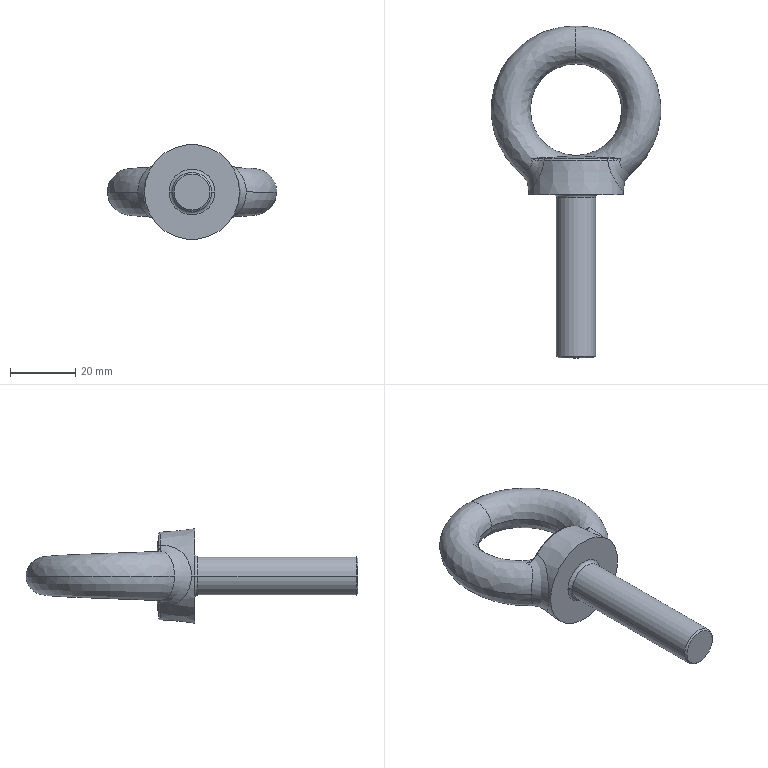Part | STEP file | GB╱T 825-1988[吊环Screw M12x50] | 1 solid | 32 faces | box 52.011 x 101.603 x 29.1 mm | volume 25092 mm3 | spline 18 | cone 6 | torus 4 | plane 2 | cylinder 2 | commonest cylinder face diameters 12 x2